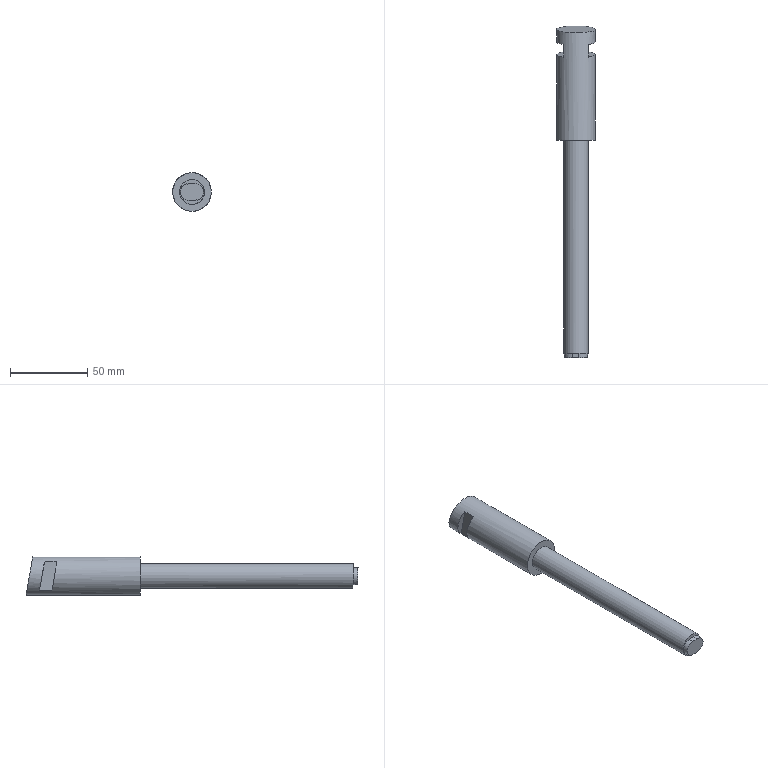Part | STEP file | solid 145 | 1 solid | 16 faces | box 25 x 214.479 x 25 mm | volume 62211 mm3 | plane 8 | spline 6 | cylinder 2 | commonest cylinder face diameters 16 x1 25 x1